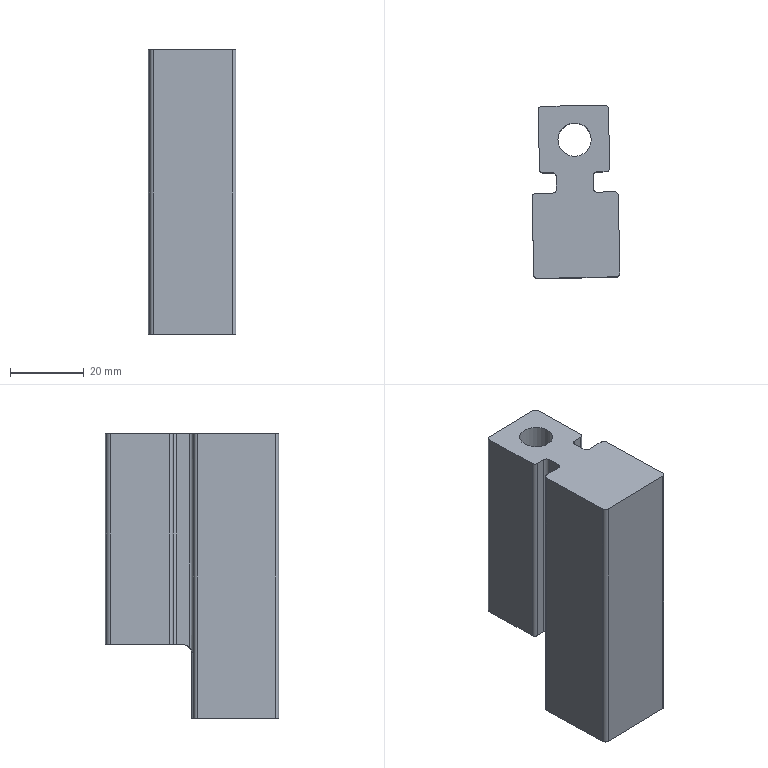Part | NX | features PU-8 2 | 1 solid | 30 faces | box 23.75 x 46.902 x 77 mm | volume 59016 mm3 | plane 15 | cylinder 15 | commonest cylinder face diameters 2 x12 6 x1 9 x1 14.5 x1
STEP:
#1=CARTESIAN_POINT('',(3034.594,-798.424,885.716));
#2=VERTEX_POINT('',#1);
#3=CARTESIAN_POINT('',(3046.592,-798.167,885.716));
#4=VERTEX_POINT('',#3);
#5=CARTESIAN_POINT('',(3046.592,-798.167,885.716));
#6=DIRECTION('',(0.9998,0.0214,0.));
#7=VECTOR('',#6,1000.);
#8=LINE('',#5,#7);
#9=EDGE_CURVE('',#2,#4,#8,.T.);
#10=ORIENTED_EDGE('',*,*,#9,.T.);
#11=CARTESIAN_POINT('',(3046.592,-798.167,945.716));
#12=VERTEX_POINT('',#11);
#13=CARTESIAN_POINT('',(3046.592,-798.167,945.716));
#14=DIRECTION('',(0.,0.,-1.));
#15=VECTOR('',#14,1000.);
#16=LINE('',#13,#15);
#17=EDGE_CURVE('',#4,#12,#16,.F.);
#18=ORIENTED_EDGE('',*,*,#17,.T.);
#19=CARTESIAN_POINT('',(3051.243,-798.068,945.716));
#20=VERTEX_POINT('',#19);
#21=CARTESIAN_POINT('',(2865.876,-802.035,945.716));
#22=DIRECTION('',(-0.9998,-0.0214,0.));
#23=VECTOR('',#22,1000.);
#24=LINE('',#21,#23);
#25=EDGE_CURVE('',#20,#12,#24,.T.);
#26=ORIENTED_EDGE('',*,*,#25,.F.);
#27=CARTESIAN_POINT('',(3051.243,-798.068,868.716));
#28=VERTEX_POINT('',#27);
#29=CARTESIAN_POINT('',(3051.243,-798.068,907.216));
#30=DIRECTION('',(0.,0.,-1.));
#31=VECTOR('',#30,1000.);
#32=LINE('',#29,#31);
#33=EDGE_CURVE('',#20,#28,#32,.T.);
#34=ORIENTED_EDGE('',*,*,#33,.T.);
#35=CARTESIAN_POINT('',(3029.943,-798.524,868.716));
#36=VERTEX_POINT('',#35);
#37=CARTESIAN_POINT('',(3028.943,-798.545,868.716));
#38=DIRECTION('',(-0.9998,-0.0214,0.));
#39=VECTOR('',#38,1000.);
#40=LINE('',#37,#39);
#41=EDGE_CURVE('',#28,#36,#40,.T.);
#42=ORIENTED_EDGE('',*,*,#41,.T.);
#43=CARTESIAN_POINT('',(3029.943,-798.524,945.716));
#44=VERTEX_POINT('',#43);
#45=CARTESIAN_POINT('',(3029.943,-798.524,907.216));
#46=DIRECTION('',(0.,0.,1.));
#47=VECTOR('',#46,1000.);
#48=LINE('',#45,#47);
#49=EDGE_CURVE('',#36,#44,#48,.T.);
#50=ORIENTED_EDGE('',*,*,#49,.T.);
#51=CARTESIAN_POINT('',(3034.594,-798.424,945.716));
#52=VERTEX_POINT('',#51);
#53=CARTESIAN_POINT('',(2865.876,-802.035,945.716));
#54=DIRECTION('',(-0.9998,-0.0214,0.));
#55=VECTOR('',#54,1000.);
#56=LINE('',#53,#55);
#57=EDGE_CURVE('',#52,#44,#56,.T.);
#58=ORIENTED_EDGE('',*,*,#57,.F.);
#59=CARTESIAN_POINT('',(3034.594,-798.424,868.716));
#60=DIRECTION('',(0.,0.,1.));
#61=VECTOR('',#60,1000.);
#62=LINE('',#59,#61);
#63=EDGE_CURVE('',#52,#2,#62,.F.);
#64=ORIENTED_EDGE('',*,*,#63,.T.);
#65=EDGE_LOOP('',(#10,#18,#26,#34,#42,#50,#58,#64));
#66=FACE_BOUND('',#65,.T.);
#67=CARTESIAN_POINT('',(3048.917,-798.117,907.216));
#68=DIRECTION('',(-0.0214,0.9998,0.));
#69=DIRECTION('',(-0.9998,-0.0214,0.));
#70=AXIS2_PLACEMENT_3D('',#67,#68,#69);
#71=PLANE('',#70);
#72=ADVANCED_FACE('',(#66),#71,.T.);
#73=CARTESIAN_POINT('',(3028.965,-799.545,868.716));
#74=VERTEX_POINT('',#73);
#75=CARTESIAN_POINT('',(3029.964,-799.523,868.716));
#76=DIRECTION('',(0.,0.,-1.));
#77=DIRECTION('',(-1.,0.,0.));
#78=AXIS2_PLACEMENT_3D('',#75,#76,#77);
#79=CIRCLE('',#78,1.);
#80=EDGE_CURVE('',#74,#36,#79,.T.);
#81=ORIENTED_EDGE('',*,*,#80,.F.);
#82=CARTESIAN_POINT('',(3028.965,-799.545,945.716));
#83=VERTEX_POINT('',#82);
#84=CARTESIAN_POINT('',(3028.965,-799.545,888.716));
#85=DIRECTION('',(0.,0.,1.));
#86=VECTOR('',#85,1000.);
#87=LINE('',#84,#86);
#88=EDGE_CURVE('',#83,#74,#87,.F.);
#89=ORIENTED_EDGE('',*,*,#88,.F.);
#90=CARTESIAN_POINT('',(3029.964,-799.523,945.716));
#91=DIRECTION('',(0.,0.,1.));
#92=DIRECTION('',(1.,0.,0.));
#93=AXIS2_PLACEMENT_3D('',#90,#91,#92);
#94=CIRCLE('',#93,1.);
#95=EDGE_CURVE('',#44,#83,#94,.T.);
#96=ORIENTED_EDGE('',*,*,#95,.F.);
#97=ORIENTED_EDGE('',*,*,#49,.F.);
#98=EDGE_LOOP('',(#81,#89,#96,#97));
#99=FACE_BOUND('',#98,.T.);
#100=CARTESIAN_POINT('',(3029.964,-799.523,907.216));
#101=DIRECTION('',(0.,0.,1.));
#102=DIRECTION('',(0.,-1.,0.));
#103=AXIS2_PLACEMENT_3D('',#100,#101,#102);
#104=CYLINDRICAL_SURFACE('',#103,1.);
#105=ADVANCED_FACE('',(#99),#104,.T.);
#106=CARTESIAN_POINT('',(3029.414,-820.542,868.716));
#107=VERTEX_POINT('',#106);
#108=CARTESIAN_POINT('',(3028.938,-798.32,868.716));
#109=DIRECTION('',(-0.0214,0.9998,0.));
#110=VECTOR('',#109,1000.);
#111=LINE('',#108,#110);
#112=EDGE_CURVE('',#107,#74,#111,.T.);
#113=ORIENTED_EDGE('',*,*,#112,.F.);
#114=CARTESIAN_POINT('',(3029.414,-820.542,945.716));
#115=VERTEX_POINT('',#114);
#116=CARTESIAN_POINT('',(3029.414,-820.542,945.716));
#117=DIRECTION('',(0.,0.,-1.));
#118=VECTOR('',#117,1000.);
#119=LINE('',#116,#118);
#120=EDGE_CURVE('',#107,#115,#119,.F.);
#121=ORIENTED_EDGE('',*,*,#120,.T.);
#122=CARTESIAN_POINT('',(3029.19,-810.082,945.716));
#123=DIRECTION('',(-0.0214,0.9998,0.));
#124=VECTOR('',#123,1000.);
#125=LINE('',#122,#124);
#126=EDGE_CURVE('',#83,#115,#125,.F.);
#127=ORIENTED_EDGE('',*,*,#126,.F.);
#128=ORIENTED_EDGE('',*,*,#88,.T.);
#129=EDGE_LOOP('',(#113,#121,#127,#128));
#130=FACE_BOUND('',#129,.T.);
#131=CARTESIAN_POINT('',(3029.19,-810.082,888.716));
#132=DIRECTION('',(-0.9998,-0.0214,0.));
#133=DIRECTION('',(0.0214,-0.9998,0.));
#134=AXIS2_PLACEMENT_3D('',#131,#132,#133);
#135=PLANE('',#134);
#136=ADVANCED_FACE('',(#130),#135,.T.);
#137=CARTESIAN_POINT('',(3030.435,-821.52,945.716));
#138=VERTEX_POINT('',#137);
#139=CARTESIAN_POINT('',(3030.414,-820.521,945.716));
#140=DIRECTION('',(0.,0.,1.));
#141=DIRECTION('',(1.,0.,0.));
#142=AXIS2_PLACEMENT_3D('',#139,#140,#141);
#143=CIRCLE('',#142,1.);
#144=EDGE_CURVE('',#115,#138,#143,.T.);
#145=ORIENTED_EDGE('',*,*,#144,.F.);
#146=ORIENTED_EDGE('',*,*,#120,.F.);
#147=CARTESIAN_POINT('',(3030.435,-821.52,868.716));
#148=VERTEX_POINT('',#147);
#149=CARTESIAN_POINT('',(3030.414,-820.521,868.716));
#150=DIRECTION('',(0.,0.,-1.));
#151=DIRECTION('',(-1.,0.,0.));
#152=AXIS2_PLACEMENT_3D('',#149,#150,#151);
#153=CIRCLE('',#152,1.);
#154=EDGE_CURVE('',#148,#107,#153,.T.);
#155=ORIENTED_EDGE('',*,*,#154,.F.);
#156=CARTESIAN_POINT('',(3030.435,-821.52,868.716));
#157=DIRECTION('',(0.,0.,-1.));
#158=VECTOR('',#157,1000.);
#159=LINE('',#156,#158);
#160=EDGE_CURVE('',#138,#148,#159,.T.);
#161=ORIENTED_EDGE('',*,*,#160,.F.);
#162=EDGE_LOOP('',(#145,#146,#155,#161));
#163=FACE_BOUND('',#162,.T.);
#164=CARTESIAN_POINT('',(3030.414,-820.521,888.716));
#165=DIRECTION('',(0.,0.,1.));
#166=DIRECTION('',(0.,-1.,0.));
#167=AXIS2_PLACEMENT_3D('',#164,#165,#166);
#168=CYLINDRICAL_SURFACE('',#167,1.);
#169=ADVANCED_FACE('',(#163),#168,.T.);
#170=CARTESIAN_POINT('',(3051.735,-821.064,868.716));
#171=VERTEX_POINT('',#170);
#172=CARTESIAN_POINT('',(3040.517,-821.305,868.716));
#173=DIRECTION('',(0.9998,0.0214,0.));
#174=VECTOR('',#173,1000.);
#175=LINE('',#172,#174);
#176=EDGE_CURVE('',#148,#171,#175,.T.);
#177=ORIENTED_EDGE('',*,*,#176,.T.);
#178=CARTESIAN_POINT('',(3051.735,-821.064,945.716));
#179=VERTEX_POINT('',#178);
#180=CARTESIAN_POINT('',(3051.735,-821.064,945.716));
#181=DIRECTION('',(0.,0.,-1.));
#182=VECTOR('',#181,1000.);
#183=LINE('',#180,#182);
#184=EDGE_CURVE('',#171,#179,#183,.F.);
#185=ORIENTED_EDGE('',*,*,#184,.T.);
#186=CARTESIAN_POINT('',(2866.368,-825.032,945.716));
#187=DIRECTION('',(-0.9998,-0.0214,0.));
#188=VECTOR('',#187,1000.);
#189=LINE('',#186,#188);
#190=EDGE_CURVE('',#138,#179,#189,.F.);
#191=ORIENTED_EDGE('',*,*,#190,.F.);
#192=ORIENTED_EDGE('',*,*,#160,.T.);
#193=EDGE_LOOP('',(#177,#185,#191,#192));
#194=FACE_BOUND('',#193,.T.);
#195=CARTESIAN_POINT('',(3029.435,-821.542,888.716));
#196=DIRECTION('',(-0.0214,0.9998,0.));
#197=DIRECTION('',(0.,0.,-1.));
#198=AXIS2_PLACEMENT_3D('',#195,#196,#197);
#199=PLANE('',#198);
#200=ADVANCED_FACE('',(#194),#199,.F.);
#201=CARTESIAN_POINT('',(3052.714,-820.043,945.716));
#202=VERTEX_POINT('',#201);
#203=CARTESIAN_POINT('',(3051.714,-820.065,945.716));
#204=DIRECTION('',(0.,0.,1.));
#205=DIRECTION('',(1.,0.,0.));
#206=AXIS2_PLACEMENT_3D('',#203,#204,#205);
#207=CIRCLE('',#206,1.);
#208=EDGE_CURVE('',#179,#202,#207,.T.);
#209=ORIENTED_EDGE('',*,*,#208,.F.);
#210=ORIENTED_EDGE('',*,*,#184,.F.);
#211=CARTESIAN_POINT('',(3052.714,-820.043,868.716));
#212=VERTEX_POINT('',#211);
#213=CARTESIAN_POINT('',(3051.714,-820.065,868.716));
#214=DIRECTION('',(0.,0.,-1.));
#215=DIRECTION('',(-1.,0.,0.));
#216=AXIS2_PLACEMENT_3D('',#213,#214,#215);
#217=CIRCLE('',#216,1.);
#218=EDGE_CURVE('',#212,#171,#217,.T.);
#219=ORIENTED_EDGE('',*,*,#218,.F.);
#220=CARTESIAN_POINT('',(3052.714,-820.043,868.716));
#221=DIRECTION('',(0.,0.,-1.));
#222=VECTOR('',#221,1000.);
#223=LINE('',#220,#222);
#224=EDGE_CURVE('',#202,#212,#223,.T.);
#225=ORIENTED_EDGE('',*,*,#224,.F.);
#226=EDGE_LOOP('',(#209,#210,#219,#225));
#227=FACE_BOUND('',#226,.T.);
#228=CARTESIAN_POINT('',(3051.714,-820.065,888.716));
#229=DIRECTION('',(0.,0.,1.));
#230=DIRECTION('',(1.,0.,0.));
#231=AXIS2_PLACEMENT_3D('',#228,#229,#230);
#232=CYLINDRICAL_SURFACE('',#231,1.);
#233=ADVANCED_FACE('',(#227),#232,.T.);
#234=CARTESIAN_POINT('',(3052.264,-799.046,868.716));
#235=VERTEX_POINT('',#234);
#236=CARTESIAN_POINT('',(3052.483,-809.276,868.716));
#237=DIRECTION('',(0.0214,-0.9998,0.));
#238=VECTOR('',#237,1000.);
#239=LINE('',#236,#238);
#240=EDGE_CURVE('',#235,#212,#239,.T.);
#241=ORIENTED_EDGE('',*,*,#240,.F.);
#242=CARTESIAN_POINT('',(3052.264,-799.046,945.716));
#243=VERTEX_POINT('',#242);
#244=CARTESIAN_POINT('',(3052.264,-799.046,888.716));
#245=DIRECTION('',(0.,0.,-1.));
#246=VECTOR('',#245,1000.);
#247=LINE('',#244,#246);
#248=EDGE_CURVE('',#235,#243,#247,.F.);
#249=ORIENTED_EDGE('',*,*,#248,.T.);
#250=CARTESIAN_POINT('',(3056.461,-995.133,945.716));
#251=DIRECTION('',(-0.0214,0.9998,0.));
#252=VECTOR('',#251,1000.);
#253=LINE('',#250,#252);
#254=EDGE_CURVE('',#243,#202,#253,.F.);
#255=ORIENTED_EDGE('',*,*,#254,.T.);
#256=ORIENTED_EDGE('',*,*,#224,.T.);
#257=EDGE_LOOP('',(#241,#249,#255,#256));
#258=FACE_BOUND('',#257,.T.);
#259=CARTESIAN_POINT('',(3052.735,-821.043,888.716));
#260=DIRECTION('',(0.9998,0.0214,0.));
#261=DIRECTION('',(0.,0.,-1.));
#262=AXIS2_PLACEMENT_3D('',#259,#260,#261);
#263=PLANE('',#262);
#264=ADVANCED_FACE('',(#258),#263,.T.);
#265=CARTESIAN_POINT('',(3051.265,-799.067,945.716));
#266=DIRECTION('',(0.,0.,1.));
#267=DIRECTION('',(1.,0.,0.));
#268=AXIS2_PLACEMENT_3D('',#265,#266,#267);
#269=CIRCLE('',#268,1.);
#270=EDGE_CURVE('',#243,#20,#269,.T.);
#271=ORIENTED_EDGE('',*,*,#270,.F.);
#272=ORIENTED_EDGE('',*,*,#248,.F.);
#273=CARTESIAN_POINT('',(3051.265,-799.067,868.716));
#274=DIRECTION('',(0.,0.,-1.));
#275=DIRECTION('',(-1.,0.,0.));
#276=AXIS2_PLACEMENT_3D('',#273,#274,#275);
#277=CIRCLE('',#276,1.);
#278=EDGE_CURVE('',#28,#235,#277,.T.);
#279=ORIENTED_EDGE('',*,*,#278,.F.);
#280=ORIENTED_EDGE('',*,*,#33,.F.);
#281=EDGE_LOOP('',(#271,#272,#279,#280));
#282=FACE_BOUND('',#281,.T.);
#283=CARTESIAN_POINT('',(3051.265,-799.067,907.216));
#284=DIRECTION('',(0.,0.,-1.));
#285=DIRECTION('',(-1.,0.,0.));
#286=AXIS2_PLACEMENT_3D('',#283,#284,#285);
#287=CYLINDRICAL_SURFACE('',#286,1.);
#288=ADVANCED_FACE('',(#282),#287,.T.);
#289=ORIENTED_EDGE('',*,*,#270,.T.);
#290=ORIENTED_EDGE('',*,*,#25,.T.);
#291=CARTESIAN_POINT('',(3045.571,-797.189,945.716));
#292=VERTEX_POINT('',#291);
#293=CARTESIAN_POINT('',(3046.57,-797.167,945.716));
#294=DIRECTION('',(0.,0.,1.));
#295=DIRECTION('',(1.,0.,0.));
#296=AXIS2_PLACEMENT_3D('',#293,#294,#295);
#297=CIRCLE('',#296,1.);
#298=EDGE_CURVE('',#12,#292,#297,.F.);
#299=ORIENTED_EDGE('',*,*,#298,.T.);
#300=CARTESIAN_POINT('',(3045.496,-793.69,945.716));
#301=VERTEX_POINT('',#300);
#302=CARTESIAN_POINT('',(3049.882,-998.642,945.716));
#303=DIRECTION('',(-0.0214,0.9998,0.));
#304=VECTOR('',#303,1000.);
#305=LINE('',#302,#304);
#306=EDGE_CURVE('',#301,#292,#305,.F.);
#307=ORIENTED_EDGE('',*,*,#306,.F.);
#308=CARTESIAN_POINT('',(3046.474,-792.668,945.716));
#309=VERTEX_POINT('',#308);
#310=CARTESIAN_POINT('',(3046.495,-793.668,945.716));
#311=DIRECTION('',(0.,0.,1.));
#312=DIRECTION('',(0.9998,0.0214,0.));
#313=AXIS2_PLACEMENT_3D('',#310,#311,#312);
#314=CIRCLE('',#313,1.);
#315=EDGE_CURVE('',#309,#301,#314,.T.);
#316=ORIENTED_EDGE('',*,*,#315,.F.);
#317=CARTESIAN_POINT('',(3048.973,-792.615,945.716));
#318=VERTEX_POINT('',#317);
#319=CARTESIAN_POINT('',(2867.193,-796.506,945.716));
#320=DIRECTION('',(0.9998,0.0214,0.));
#321=VECTOR('',#320,1000.);
#322=LINE('',#319,#321);
#323=EDGE_CURVE('',#318,#309,#322,.F.);
#324=ORIENTED_EDGE('',*,*,#323,.F.);
#325=CARTESIAN_POINT('',(3049.952,-791.594,945.716));
#326=VERTEX_POINT('',#325);
#327=CARTESIAN_POINT('',(3048.952,-791.615,945.716));
#328=DIRECTION('',(0.,0.,1.));
#329=DIRECTION('',(0.9998,0.0214,0.));
#330=AXIS2_PLACEMENT_3D('',#327,#328,#329);
#331=CIRCLE('',#330,1.);
#332=EDGE_CURVE('',#326,#318,#331,.F.);
#333=ORIENTED_EDGE('',*,*,#332,.F.);
#334=CARTESIAN_POINT('',(3049.609,-775.597,945.716));
#335=VERTEX_POINT('',#334);
#336=CARTESIAN_POINT('',(3054.392,-999.046,945.716));
#337=DIRECTION('',(-0.0214,0.9998,0.));
#338=VECTOR('',#337,1000.);
#339=LINE('',#336,#338);
#340=EDGE_CURVE('',#335,#326,#339,.F.);
#341=ORIENTED_EDGE('',*,*,#340,.F.);
#342=CARTESIAN_POINT('',(3048.588,-774.619,945.716));
#343=VERTEX_POINT('',#342);
#344=CARTESIAN_POINT('',(3048.61,-775.619,945.716));
#345=DIRECTION('',(0.,0.,1.));
#346=DIRECTION('',(0.9998,0.0214,0.));
#347=AXIS2_PLACEMENT_3D('',#344,#345,#346);
#348=CIRCLE('',#347,1.);
#349=EDGE_CURVE('',#343,#335,#348,.F.);
#350=ORIENTED_EDGE('',*,*,#349,.F.);
#351=CARTESIAN_POINT('',(3031.592,-774.983,945.716));
#352=VERTEX_POINT('',#351);
#353=CARTESIAN_POINT('',(2866.808,-778.51,945.716));
#354=DIRECTION('',(-0.9998,-0.0214,0.));
#355=VECTOR('',#354,1000.);
#356=LINE('',#353,#355);
#357=EDGE_CURVE('',#352,#343,#356,.F.);
#358=ORIENTED_EDGE('',*,*,#357,.F.);
#359=CARTESIAN_POINT('',(3030.614,-776.004,945.716));
#360=VERTEX_POINT('',#359);
#361=CARTESIAN_POINT('',(3031.614,-775.983,945.716));
#362=DIRECTION('',(0.,0.,1.));
#363=DIRECTION('',(0.9998,0.0214,0.));
#364=AXIS2_PLACEMENT_3D('',#361,#362,#363);
#365=CIRCLE('',#364,1.);
#366=EDGE_CURVE('',#360,#352,#365,.F.);
#367=ORIENTED_EDGE('',*,*,#366,.F.);
#368=CARTESIAN_POINT('',(3030.956,-792.,945.716));
#369=VERTEX_POINT('',#368);
#370=CARTESIAN_POINT('',(3035.396,-999.452,945.716));
#371=DIRECTION('',(0.0214,-0.9998,0.));
#372=VECTOR('',#371,1000.);
#373=LINE('',#370,#372);
#374=EDGE_CURVE('',#369,#360,#373,.F.);
#375=ORIENTED_EDGE('',*,*,#374,.F.);
#376=CARTESIAN_POINT('',(3031.977,-792.979,945.716));
#377=VERTEX_POINT('',#376);
#378=CARTESIAN_POINT('',(3031.956,-791.979,945.716));
#379=DIRECTION('',(0.,0.,1.));
#380=DIRECTION('',(0.9998,0.0214,0.));
#381=AXIS2_PLACEMENT_3D('',#378,#379,#380);
#382=CIRCLE('',#381,1.);
#383=EDGE_CURVE('',#377,#369,#382,.F.);
#384=ORIENTED_EDGE('',*,*,#383,.F.);
#385=CARTESIAN_POINT('',(3034.477,-792.925,945.716));
#386=VERTEX_POINT('',#385);
#387=CARTESIAN_POINT('',(2867.193,-796.506,945.716));
#388=DIRECTION('',(0.9998,0.0214,0.));
#389=VECTOR('',#388,1000.);
#390=LINE('',#387,#389);
#391=EDGE_CURVE('',#386,#377,#390,.F.);
#392=ORIENTED_EDGE('',*,*,#391,.F.);
#393=CARTESIAN_POINT('',(3035.498,-793.904,945.716));
#394=VERTEX_POINT('',#393);
#395=CARTESIAN_POINT('',(3034.498,-793.925,945.716));
#396=DIRECTION('',(0.,0.,1.));
#397=DIRECTION('',(0.9998,0.0214,0.));
#398=AXIS2_PLACEMENT_3D('',#395,#396,#397);
#399=CIRCLE('',#398,1.);
#400=EDGE_CURVE('',#394,#386,#399,.T.);
#401=ORIENTED_EDGE('',*,*,#400,.F.);
#402=CARTESIAN_POINT('',(3035.573,-797.403,945.716));
#403=VERTEX_POINT('',#402);
#404=CARTESIAN_POINT('',(3039.884,-998.856,945.716));
#405=DIRECTION('',(0.0214,-0.9998,0.));
#406=VECTOR('',#405,1000.);
#407=LINE('',#404,#406);
#408=EDGE_CURVE('',#403,#394,#407,.F.);
#409=ORIENTED_EDGE('',*,*,#408,.F.);
#410=CARTESIAN_POINT('',(3034.573,-797.424,945.716));
#411=DIRECTION('',(0.,0.,1.));
#412=DIRECTION('',(1.,0.,0.));
#413=AXIS2_PLACEMENT_3D('',#410,#411,#412);
#414=CIRCLE('',#413,1.);
#415=EDGE_CURVE('',#403,#52,#414,.F.);
#416=ORIENTED_EDGE('',*,*,#415,.T.);
#417=ORIENTED_EDGE('',*,*,#57,.T.);
#418=ORIENTED_EDGE('',*,*,#95,.T.);
#419=ORIENTED_EDGE('',*,*,#126,.T.);
#420=ORIENTED_EDGE('',*,*,#144,.T.);
#421=ORIENTED_EDGE('',*,*,#190,.T.);
#422=ORIENTED_EDGE('',*,*,#208,.T.);
#423=ORIENTED_EDGE('',*,*,#254,.F.);
#424=EDGE_LOOP('',(#289,#290,#299,#307,#316,#324,#333,#341,#350,#358,#367,#375,#384,#392,#401,#409,#416,#417,#418,#419,#420,#421,#422,#423));
#425=FACE_BOUND('',#424,.T.);
#426=CARTESIAN_POINT('',(3044.952,-783.979,945.716));
#427=VERTEX_POINT('',#426);
#428=CARTESIAN_POINT('',(3040.452,-783.979,945.716));
#429=DIRECTION('',(0.,0.,1.));
#430=DIRECTION('',(1.,0.,0.));
#431=AXIS2_PLACEMENT_3D('',#428,#429,#430);
#432=CIRCLE('',#431,4.5);
#433=EDGE_CURVE('',#427,#427,#432,.F.);
#434=ORIENTED_EDGE('',*,*,#433,.T.);
#435=EDGE_LOOP('',(#434));
#436=FACE_BOUND('',#435,.T.);
#437=CARTESIAN_POINT('',(2870.094,-999.122,945.716));
#438=DIRECTION('',(0.,0.,1.));
#439=DIRECTION('',(0.,1.,0.));
#440=AXIS2_PLACEMENT_3D('',#437,#438,#439);
#441=PLANE('',#440);
#442=ADVANCED_FACE('',(#425,#436),#441,.T.);
#443=ORIENTED_EDGE('',*,*,#41,.F.);
#444=ORIENTED_EDGE('',*,*,#278,.T.);
#445=ORIENTED_EDGE('',*,*,#240,.T.);
#446=ORIENTED_EDGE('',*,*,#218,.T.);
#447=ORIENTED_EDGE('',*,*,#176,.F.);
#448=ORIENTED_EDGE('',*,*,#154,.T.);
#449=ORIENTED_EDGE('',*,*,#112,.T.);
#450=ORIENTED_EDGE('',*,*,#80,.T.);
#451=EDGE_LOOP('',(#443,#444,#445,#446,#447,#448,#449,#450));
#452=FACE_BOUND('',#451,.T.);
#453=CARTESIAN_POINT('',(3040.266,-809.538,868.716));
#454=DIRECTION('',(0.,0.,-1.));
#455=DIRECTION('',(-0.0349,0.9994,0.));
#456=AXIS2_PLACEMENT_3D('',#453,#454,#455);
#457=PLANE('',#456);
#458=ADVANCED_FACE('',(#452),#457,.T.);
#459=ORIENTED_EDGE('',*,*,#306,.T.);
#460=CARTESIAN_POINT('',(3045.571,-797.189,887.952));
#461=VERTEX_POINT('',#460);
#462=CARTESIAN_POINT('',(3045.571,-797.189,868.716));
#463=DIRECTION('',(0.,0.,-1.));
#464=VECTOR('',#463,1000.);
#465=LINE('',#462,#464);
#466=EDGE_CURVE('',#292,#461,#465,.T.);
#467=ORIENTED_EDGE('',*,*,#466,.T.);
#468=CARTESIAN_POINT('',(3045.528,-795.189,888.716));
#469=VERTEX_POINT('',#468);
#470=CARTESIAN_POINT('',(3045.528,-795.189,885.716));
#471=DIRECTION('',(0.9998,0.0214,0.));
#472=DIRECTION('',(-0.0214,0.9998,0.));
#473=AXIS2_PLACEMENT_3D('',#470,#471,#472);
#474=CIRCLE('',#473,3.);
#475=EDGE_CURVE('',#461,#469,#474,.F.);
#476=ORIENTED_EDGE('',*,*,#475,.T.);
#477=CARTESIAN_POINT('',(3045.496,-793.69,888.716));
#478=VERTEX_POINT('',#477);
#479=CARTESIAN_POINT('',(3045.832,-809.419,888.716));
#480=DIRECTION('',(0.0214,-0.9998,0.));
#481=VECTOR('',#480,1000.);
#482=LINE('',#479,#481);
#483=EDGE_CURVE('',#478,#469,#482,.T.);
#484=ORIENTED_EDGE('',*,*,#483,.F.);
#485=CARTESIAN_POINT('',(3045.496,-793.69,900.716));
#486=DIRECTION('',(0.,0.,-1.));
#487=VECTOR('',#486,1000.);
#488=LINE('',#485,#487);
#489=EDGE_CURVE('',#301,#478,#488,.T.);
#490=ORIENTED_EDGE('',*,*,#489,.F.);
#491=EDGE_LOOP('',(#459,#467,#476,#484,#490));
#492=FACE_BOUND('',#491,.T.);
#493=CARTESIAN_POINT('',(3045.485,-793.19,900.716));
#494=DIRECTION('',(0.9998,0.0214,0.));
#495=DIRECTION('',(-0.0214,0.9998,0.));
#496=AXIS2_PLACEMENT_3D('',#493,#494,#495);
#497=PLANE('',#496);
#498=ADVANCED_FACE('',(#492),#497,.T.);
#499=ORIENTED_EDGE('',*,*,#298,.F.);
#500=ORIENTED_EDGE('',*,*,#17,.F.);
#501=CARTESIAN_POINT('',(3045.571,-797.189,887.952));
#502=CARTESIAN_POINT('',(3045.578,-797.534,887.644));
#503=CARTESIAN_POINT('',(3045.906,-798.032,886.9));
#504=CARTESIAN_POINT('',(3046.363,-798.172,886.113));
#505=CARTESIAN_POINT('',(3046.592,-798.167,885.716));
#506=B_SPLINE_CURVE_WITH_KNOTS('',3,(#501,#502,#503,#504,#505),.UNSPECIFIED.,.F.,.F.,(4,1,4),(0.,0.001374,0.002748),.UNSPECIFIED.);
#507=EDGE_CURVE('',#4,#461,#506,.F.);
#508=ORIENTED_EDGE('',*,*,#507,.T.);
#509=ORIENTED_EDGE('',*,*,#466,.F.);
#510=EDGE_LOOP('',(#499,#500,#508,#509));
#511=FACE_BOUND('',#510,.T.);
#512=CARTESIAN_POINT('',(3046.57,-797.167,900.716));
#513=DIRECTION('',(0.,0.,1.));
#514=DIRECTION('',(1.,0.,0.));
#515=AXIS2_PLACEMENT_3D('',#512,#513,#514);
#516=CYLINDRICAL_SURFACE('',#515,1.);
#517=ADVANCED_FACE('',(#511),#516,.F.);
#518=CARTESIAN_POINT('',(3035.573,-797.403,887.952));
#519=VERTEX_POINT('',#518);
#520=CARTESIAN_POINT('',(3035.573,-797.403,945.716));
#521=DIRECTION('',(0.,0.,1.));
#522=VECTOR('',#521,1000.);
#523=LINE('',#520,#522);
#524=EDGE_CURVE('',#519,#403,#523,.T.);
#525=ORIENTED_EDGE('',*,*,#524,.F.);
#526=CARTESIAN_POINT('',(3035.573,-797.403,887.952));
#527=CARTESIAN_POINT('',(3035.58,-797.748,887.644));
#528=CARTESIAN_POINT('',(3035.274,-798.259,886.9));
#529=CARTESIAN_POINT('',(3034.823,-798.419,886.113));
#530=CARTESIAN_POINT('',(3034.594,-798.424,885.716));
#531=B_SPLINE_CURVE_WITH_KNOTS('',3,(#526,#527,#528,#529,#530),.UNSPECIFIED.,.F.,.F.,(4,1,4),(0.,0.001374,0.002748),.UNSPECIFIED.);
#532=EDGE_CURVE('',#519,#2,#531,.T.);
#533=ORIENTED_EDGE('',*,*,#532,.T.);
#534=ORIENTED_EDGE('',*,*,#63,.F.);
#535=ORIENTED_EDGE('',*,*,#415,.F.);
#536=EDGE_LOOP('',(#525,#533,#534,#535));
#537=FACE_BOUND('',#536,.T.);
#538=CARTESIAN_POINT('',(3034.573,-797.424,900.716));
#539=DIRECTION('',(0.,0.,-1.));
#540=DIRECTION('',(-1.,0.,0.));
#541=AXIS2_PLACEMENT_3D('',#538,#539,#540);
#542=CYLINDRICAL_SURFACE('',#541,1.);
#543=ADVANCED_FACE('',(#537),#542,.F.);
#544=CARTESIAN_POINT('',(3035.53,-795.403,888.716));
#545=VERTEX_POINT('',#544);
#546=CARTESIAN_POINT('',(3035.498,-793.904,888.716));
#547=VERTEX_POINT('',#546);
#548=CARTESIAN_POINT('',(3035.835,-809.633,888.716));
#549=DIRECTION('',(-0.0214,0.9998,0.));
#550=VECTOR('',#549,1000.);
#551=LINE('',#548,#550);
#552=EDGE_CURVE('',#545,#547,#551,.T.);
#553=ORIENTED_EDGE('',*,*,#552,.F.);
#554=CARTESIAN_POINT('',(3035.53,-795.403,885.716));
#555=DIRECTION('',(-0.9998,-0.0214,0.));
#556=DIRECTION('',(0.0214,-0.9998,0.));
#557=AXIS2_PLACEMENT_3D('',#554,#555,#556);
#558=CIRCLE('',#557,3.);
#559=EDGE_CURVE('',#545,#519,#558,.F.);
#560=ORIENTED_EDGE('',*,*,#559,.T.);
#561=ORIENTED_EDGE('',*,*,#524,.T.);
#562=ORIENTED_EDGE('',*,*,#408,.T.);
#563=CARTESIAN_POINT('',(3035.498,-793.904,900.716));
#564=DIRECTION('',(0.,0.,1.));
#565=VECTOR('',#564,1000.);
#566=LINE('',#563,#565);
#567=EDGE_CURVE('',#394,#547,#566,.F.);
#568=ORIENTED_EDGE('',*,*,#567,.T.);
#569=EDGE_LOOP('',(#553,#560,#561,#562,#568));
#570=FACE_BOUND('',#569,.T.);
#571=CARTESIAN_POINT('',(3035.573,-797.403,900.716));
#572=DIRECTION('',(-0.9998,-0.0214,0.));
#573=DIRECTION('',(0.0214,-0.9998,0.));
#574=AXIS2_PLACEMENT_3D('',#571,#572,#573);
#575=PLANE('',#574);
#576=ADVANCED_FACE('',(#570),#575,.T.);
#577=ORIENTED_EDGE('',*,*,#483,.T.);
#578=CARTESIAN_POINT('',(3034.53,-795.425,888.716));
#579=DIRECTION('',(0.9998,0.0214,0.));
#580=VECTOR('',#579,1000.);
#581=LINE('',#578,#580);
#582=EDGE_CURVE('',#469,#545,#581,.F.);
#583=ORIENTED_EDGE('',*,*,#582,.T.);
#584=ORIENTED_EDGE('',*,*,#552,.T.);
#585=CARTESIAN_POINT('',(3034.477,-792.925,888.716));
#586=VERTEX_POINT('',#585);
#587=CARTESIAN_POINT('',(3034.498,-793.925,888.716));
#588=DIRECTION('',(0.,0.,-1.));
#589=DIRECTION('',(-1.,0.,0.));
#590=AXIS2_PLACEMENT_3D('',#587,#588,#589);
#591=CIRCLE('',#590,1.);
#592=EDGE_CURVE('',#547,#586,#591,.F.);
#593=ORIENTED_EDGE('',*,*,#592,.T.);
#594=CARTESIAN_POINT('',(3031.977,-792.979,888.716));
#595=VERTEX_POINT('',#594);
#596=CARTESIAN_POINT('',(3039.908,-792.809,888.716));
#597=DIRECTION('',(-0.9998,-0.0214,0.));
#598=VECTOR('',#597,1000.);
#599=LINE('',#596,#598);
#600=EDGE_CURVE('',#586,#595,#599,.T.);
#601=ORIENTED_EDGE('',*,*,#600,.T.);
#602=CARTESIAN_POINT('',(3030.956,-792.,888.716));
#603=VERTEX_POINT('',#602);
#604=CARTESIAN_POINT('',(3031.956,-791.979,888.716));
#605=DIRECTION('',(0.,0.,-1.));
#606=DIRECTION('',(-1.,0.,0.));
#607=AXIS2_PLACEMENT_3D('',#604,#605,#606);
#608=CIRCLE('',#607,1.);
#609=EDGE_CURVE('',#595,#603,#608,.T.);
#610=ORIENTED_EDGE('',*,*,#609,.T.);
#611=CARTESIAN_POINT('',(3030.614,-776.004,888.716));
#612=VERTEX_POINT('',#611);
#613=CARTESIAN_POINT('',(3031.336,-809.729,888.716));
#614=DIRECTION('',(-0.0214,0.9998,0.));
#615=VECTOR('',#614,1000.);
#616=LINE('',#613,#615);
#617=EDGE_CURVE('',#603,#612,#616,.T.);
#618=ORIENTED_EDGE('',*,*,#617,.T.);
#619=CARTESIAN_POINT('',(3031.592,-774.983,888.716));
#620=VERTEX_POINT('',#619);
#621=CARTESIAN_POINT('',(3031.614,-775.983,888.716));
#622=DIRECTION('',(0.,0.,-1.));
#623=DIRECTION('',(-1.,0.,0.));
#624=AXIS2_PLACEMENT_3D('',#621,#622,#623);
#625=CIRCLE('',#624,1.);
#626=EDGE_CURVE('',#612,#620,#625,.T.);
#627=ORIENTED_EDGE('',*,*,#626,.T.);
#628=CARTESIAN_POINT('',(3048.588,-774.619,888.716));
#629=VERTEX_POINT('',#628);
#630=CARTESIAN_POINT('',(3039.522,-774.813,888.716));
#631=DIRECTION('',(0.9998,0.0214,0.));
#632=VECTOR('',#631,1000.);
#633=LINE('',#630,#632);
#634=EDGE_CURVE('',#620,#629,#633,.T.);
#635=ORIENTED_EDGE('',*,*,#634,.T.);
#636=CARTESIAN_POINT('',(3049.609,-775.597,888.716));
#637=VERTEX_POINT('',#636);
#638=CARTESIAN_POINT('',(3048.61,-775.619,888.716));
#639=DIRECTION('',(0.,0.,-1.));
#640=DIRECTION('',(-1.,0.,0.));
#641=AXIS2_PLACEMENT_3D('',#638,#639,#640);
#642=CIRCLE('',#641,1.);
#643=EDGE_CURVE('',#629,#637,#642,.T.);
#644=ORIENTED_EDGE('',*,*,#643,.T.);
#645=CARTESIAN_POINT('',(3049.952,-791.594,888.716));
#646=VERTEX_POINT('',#645);
#647=CARTESIAN_POINT('',(3050.331,-809.323,888.716));
#648=DIRECTION('',(0.0214,-0.9998,0.));
#649=VECTOR('',#648,1000.);
#650=LINE('',#647,#649);
#651=EDGE_CURVE('',#637,#646,#650,.T.);
#652=ORIENTED_EDGE('',*,*,#651,.T.);
#653=CARTESIAN_POINT('',(3048.973,-792.615,888.716));
#654=VERTEX_POINT('',#653);
#655=CARTESIAN_POINT('',(3048.952,-791.615,888.716));
#656=DIRECTION('',(0.,0.,-1.));
#657=DIRECTION('',(-1.,0.,0.));
#658=AXIS2_PLACEMENT_3D('',#655,#656,#657);
#659=CIRCLE('',#658,1.);
#660=EDGE_CURVE('',#646,#654,#659,.T.);
#661=ORIENTED_EDGE('',*,*,#660,.T.);
#662=CARTESIAN_POINT('',(3046.474,-792.668,888.716));
#663=VERTEX_POINT('',#662);
#664=CARTESIAN_POINT('',(3039.908,-792.809,888.716));
#665=DIRECTION('',(-0.9998,-0.0214,0.));
#666=VECTOR('',#665,1000.);
#667=LINE('',#664,#666);
#668=EDGE_CURVE('',#654,#663,#667,.T.);
#669=ORIENTED_EDGE('',*,*,#668,.T.);
#670=CARTESIAN_POINT('',(3046.495,-793.668,888.716));
#671=DIRECTION('',(0.,0.,-1.));
#672=DIRECTION('',(-1.,0.,0.));
#673=AXIS2_PLACEMENT_3D('',#670,#671,#672);
#674=CIRCLE('',#673,1.);
#675=EDGE_CURVE('',#663,#478,#674,.F.);
#676=ORIENTED_EDGE('',*,*,#675,.T.);
#677=EDGE_LOOP('',(#577,#583,#584,#593,#601,#610,#618,#627,#635,#644,#652,#661,#669,#676));
#678=FACE_BOUND('',#677,.T.);
#679=CARTESIAN_POINT('',(3033.202,-783.979,888.716));
#680=VERTEX_POINT('',#679);
#681=CARTESIAN_POINT('',(3040.452,-783.979,888.716));
#682=DIRECTION('',(0.,0.,-1.));
#683=DIRECTION('',(-1.,0.,0.));
#684=AXIS2_PLACEMENT_3D('',#681,#682,#683);
#685=CIRCLE('',#684,7.25);
#686=EDGE_CURVE('',#680,#680,#685,.T.);
#687=ORIENTED_EDGE('',*,*,#686,.F.);
#688=EDGE_LOOP('',(#687));
#689=FACE_BOUND('',#688,.T.);
#690=CARTESIAN_POINT('',(3040.266,-809.538,888.716));
#691=DIRECTION('',(0.,0.,-1.));
#692=DIRECTION('',(-0.0349,0.9994,0.));
#693=AXIS2_PLACEMENT_3D('',#690,#691,#692);
#694=PLANE('',#693);
#695=ADVANCED_FACE('',(#678,#689),#694,.T.);
#696=ORIENTED_EDGE('',*,*,#592,.F.);
#697=ORIENTED_EDGE('',*,*,#567,.F.);
#698=ORIENTED_EDGE('',*,*,#400,.T.);
#699=CARTESIAN_POINT('',(3034.477,-792.925,900.716));
#700=DIRECTION('',(0.,0.,-1.));
#701=VECTOR('',#700,1000.);
#702=LINE('',#699,#701);
#703=EDGE_CURVE('',#386,#586,#702,.T.);
#704=ORIENTED_EDGE('',*,*,#703,.T.);
#705=EDGE_LOOP('',(#696,#697,#698,#704));
#706=FACE_BOUND('',#705,.T.);
#707=CARTESIAN_POINT('',(3034.498,-793.925,900.716));
#708=DIRECTION('',(0.,0.,-1.));
#709=DIRECTION('',(-0.0135,-0.9999,0.));
#710=AXIS2_PLACEMENT_3D('',#707,#708,#709);
#711=CYLINDRICAL_SURFACE('',#710,1.);
#712=ADVANCED_FACE('',(#706),#711,.F.);
#713=ORIENTED_EDGE('',*,*,#675,.F.);
#714=CARTESIAN_POINT('',(3046.474,-792.668,900.716));
#715=DIRECTION('',(0.,0.,-1.));
#716=VECTOR('',#715,1000.);
#717=LINE('',#714,#716);
#718=EDGE_CURVE('',#309,#663,#717,.T.);
#719=ORIENTED_EDGE('',*,*,#718,.F.);
#720=ORIENTED_EDGE('',*,*,#315,.T.);
#721=ORIENTED_EDGE('',*,*,#489,.T.);
#722=EDGE_LOOP('',(#713,#719,#720,#721));
#723=FACE_BOUND('',#722,.T.);
#724=CARTESIAN_POINT('',(3046.495,-793.668,900.716));
#725=DIRECTION('',(0.,0.,-1.));
#726=DIRECTION('',(-0.0135,-0.9999,0.));
#727=AXIS2_PLACEMENT_3D('',#724,#725,#726);
#728=CYLINDRICAL_SURFACE('',#727,1.);
#729=ADVANCED_FACE('',(#723),#728,.F.);
#730=ORIENTED_EDGE('',*,*,#703,.F.);
#731=ORIENTED_EDGE('',*,*,#391,.T.);
#732=CARTESIAN_POINT('',(3031.977,-792.979,900.716));
#733=DIRECTION('',(0.,0.,-1.));
#734=VECTOR('',#733,1000.);
#735=LINE('',#732,#734);
#736=EDGE_CURVE('',#377,#595,#735,.T.);
#737=ORIENTED_EDGE('',*,*,#736,.T.);
#738=ORIENTED_EDGE('',*,*,#600,.F.);
#739=EDGE_LOOP('',(#730,#731,#737,#738));
#740=FACE_BOUND('',#739,.T.);
#741=CARTESIAN_POINT('',(3050.473,-792.583,900.716));
#742=DIRECTION('',(0.0214,-0.9998,0.));
#743=DIRECTION('',(0.9998,0.0214,0.));
#744=AXIS2_PLACEMENT_3D('',#741,#742,#743);
#745=PLANE('',#744);
#746=ADVANCED_FACE('',(#740),#745,.T.);
#747=ORIENTED_EDGE('',*,*,#626,.F.);
#748=CARTESIAN_POINT('',(3030.614,-776.004,900.716));
#749=DIRECTION('',(0.,0.,-1.));
#750=VECTOR('',#749,1000.);
#751=LINE('',#748,#750);
#752=EDGE_CURVE('',#360,#612,#751,.T.);
#753=ORIENTED_EDGE('',*,*,#752,.F.);
#754=ORIENTED_EDGE('',*,*,#366,.T.);
#755=CARTESIAN_POINT('',(3031.592,-774.983,900.716));
#756=DIRECTION('',(0.,0.,-1.));
#757=VECTOR('',#756,1000.);
#758=LINE('',#755,#757);
#759=EDGE_CURVE('',#352,#620,#758,.T.);
#760=ORIENTED_EDGE('',*,*,#759,.T.);
#761=EDGE_LOOP('',(#747,#753,#754,#760));
#762=FACE_BOUND('',#761,.T.);
#763=CARTESIAN_POINT('',(3031.614,-775.983,900.716));
#764=DIRECTION('',(0.,0.,-1.));
#765=DIRECTION('',(-0.0135,-0.9999,0.));
#766=AXIS2_PLACEMENT_3D('',#763,#764,#765);
#767=CYLINDRICAL_SURFACE('',#766,1.);
#768=ADVANCED_FACE('',(#762),#767,.T.);
#769=ORIENTED_EDGE('',*,*,#634,.F.);
#770=ORIENTED_EDGE('',*,*,#759,.F.);
#771=ORIENTED_EDGE('',*,*,#357,.T.);
#772=CARTESIAN_POINT('',(3048.588,-774.619,900.716));
#773=DIRECTION('',(0.,0.,-1.));
#774=VECTOR('',#773,1000.);
#775=LINE('',#772,#774);
#776=EDGE_CURVE('',#343,#629,#775,.T.);
#777=ORIENTED_EDGE('',*,*,#776,.T.);
#778=EDGE_LOOP('',(#769,#770,#771,#777));
#779=FACE_BOUND('',#778,.T.);
#780=CARTESIAN_POINT('',(3030.093,-775.015,900.716));
#781=DIRECTION('',(-0.0214,0.9998,0.));
#782=DIRECTION('',(-0.9998,-0.0214,0.));
#783=AXIS2_PLACEMENT_3D('',#780,#781,#782);
#784=PLANE('',#783);
#785=ADVANCED_FACE('',(#779),#784,.T.);
#786=ORIENTED_EDGE('',*,*,#643,.F.);
#787=ORIENTED_EDGE('',*,*,#776,.F.);
#788=ORIENTED_EDGE('',*,*,#349,.T.);
#789=CARTESIAN_POINT('',(3049.609,-775.597,900.716));
#790=DIRECTION('',(0.,0.,-1.));
#791=VECTOR('',#790,1000.);
#792=LINE('',#789,#791);
#793=EDGE_CURVE('',#335,#637,#792,.T.);
#794=ORIENTED_EDGE('',*,*,#793,.T.);
#795=EDGE_LOOP('',(#786,#787,#788,#794));
#796=FACE_BOUND('',#795,.T.);
#797=CARTESIAN_POINT('',(3048.61,-775.619,900.716));
#798=DIRECTION('',(0.,0.,-1.));
#799=DIRECTION('',(-0.0135,-0.9999,0.));
#800=AXIS2_PLACEMENT_3D('',#797,#798,#799);
#801=CYLINDRICAL_SURFACE('',#800,1.);
#802=ADVANCED_FACE('',(#796),#801,.T.);
#803=ORIENTED_EDGE('',*,*,#651,.F.);
#804=ORIENTED_EDGE('',*,*,#793,.F.);
#805=ORIENTED_EDGE('',*,*,#340,.T.);
#806=CARTESIAN_POINT('',(3049.952,-791.594,900.716));
#807=DIRECTION('',(0.,0.,-1.));
#808=VECTOR('',#807,1000.);
#809=LINE('',#806,#808);
#810=EDGE_CURVE('',#326,#646,#809,.T.);
#811=ORIENTED_EDGE('',*,*,#810,.T.);
#812=EDGE_LOOP('',(#803,#804,#805,#811));
#813=FACE_BOUND('',#812,.T.);
#814=CARTESIAN_POINT('',(3049.866,-787.595,900.716));
#815=DIRECTION('',(0.9998,0.0214,0.));
#816=DIRECTION('',(-0.0214,0.9998,0.));
#817=AXIS2_PLACEMENT_3D('',#814,#815,#816);
#818=PLANE('',#817);
#819=ADVANCED_FACE('',(#813),#818,.T.);
#820=ORIENTED_EDGE('',*,*,#660,.F.);
#821=ORIENTED_EDGE('',*,*,#810,.F.);
#822=ORIENTED_EDGE('',*,*,#332,.T.);
#823=CARTESIAN_POINT('',(3048.973,-792.615,900.716));
#824=DIRECTION('',(0.,0.,-1.));
#825=VECTOR('',#824,1000.);
#826=LINE('',#823,#825);
#827=EDGE_CURVE('',#318,#654,#826,.T.);
#828=ORIENTED_EDGE('',*,*,#827,.T.);
#829=EDGE_LOOP('',(#820,#821,#822,#828));
#830=FACE_BOUND('',#829,.T.);
#831=CARTESIAN_POINT('',(3048.952,-791.615,900.716));
#832=DIRECTION('',(0.,0.,-1.));
#833=DIRECTION('',(-0.0135,-0.9999,0.));
#834=AXIS2_PLACEMENT_3D('',#831,#832,#833);
#835=CYLINDRICAL_SURFACE('',#834,1.);
#836=ADVANCED_FACE('',(#830),#835,.T.);
#837=ORIENTED_EDGE('',*,*,#323,.T.);
#838=ORIENTED_EDGE('',*,*,#718,.T.);
#839=ORIENTED_EDGE('',*,*,#668,.F.);
#840=ORIENTED_EDGE('',*,*,#827,.F.);
#841=EDGE_LOOP('',(#837,#838,#839,#840));
#842=FACE_BOUND('',#841,.T.);
#843=CARTESIAN_POINT('',(3050.473,-792.583,900.716));
#844=DIRECTION('',(0.0214,-0.9998,0.));
#845=DIRECTION('',(0.9998,0.0214,0.));
#846=AXIS2_PLACEMENT_3D('',#843,#844,#845);
#847=PLANE('',#846);
#848=ADVANCED_FACE('',(#842),#847,.T.);
#849=ORIENTED_EDGE('',*,*,#609,.F.);
#850=ORIENTED_EDGE('',*,*,#736,.F.);
#851=ORIENTED_EDGE('',*,*,#383,.T.);
#852=CARTESIAN_POINT('',(3030.956,-792.,900.716));
#853=DIRECTION('',(0.,0.,-1.));
#854=VECTOR('',#853,1000.);
#855=LINE('',#852,#854);
#856=EDGE_CURVE('',#369,#603,#855,.T.);
#857=ORIENTED_EDGE('',*,*,#856,.T.);
#858=EDGE_LOOP('',(#849,#850,#851,#857));
#859=FACE_BOUND('',#858,.T.);
#860=CARTESIAN_POINT('',(3031.956,-791.979,900.716));
#861=DIRECTION('',(0.,0.,-1.));
#862=DIRECTION('',(-0.0135,-0.9999,0.));
#863=AXIS2_PLACEMENT_3D('',#860,#861,#862);
#864=CYLINDRICAL_SURFACE('',#863,1.);
#865=ADVANCED_FACE('',(#859),#864,.T.);
#866=ORIENTED_EDGE('',*,*,#617,.F.);
#867=ORIENTED_EDGE('',*,*,#856,.F.);
#868=ORIENTED_EDGE('',*,*,#374,.T.);
#869=ORIENTED_EDGE('',*,*,#752,.T.);
#870=EDGE_LOOP('',(#866,#867,#868,#869));
#871=FACE_BOUND('',#870,.T.);
#872=CARTESIAN_POINT('',(3030.956,-792.,900.716));
#873=DIRECTION('',(-0.9998,-0.0214,0.));
#874=DIRECTION('',(0.0214,-0.9998,0.));
#875=AXIS2_PLACEMENT_3D('',#872,#873,#874);
#876=PLANE('',#875);
#877=ADVANCED_FACE('',(#871),#876,.T.);
#878=CARTESIAN_POINT('',(3035.952,-783.979,900.716));
#879=VERTEX_POINT('',#878);
#880=CARTESIAN_POINT('',(3040.452,-783.979,900.716));
#881=DIRECTION('',(0.,0.,-1.));
#882=DIRECTION('',(-1.,0.,0.));
#883=AXIS2_PLACEMENT_3D('',#880,#881,#882);
#884=CIRCLE('',#883,4.5);
#885=EDGE_CURVE('',#879,#879,#884,.T.);
#886=ORIENTED_EDGE('',*,*,#885,.T.);
#887=EDGE_LOOP('',(#886));
#888=FACE_BOUND('',#887,.T.);
#889=ORIENTED_EDGE('',*,*,#433,.F.);
#890=EDGE_LOOP('',(#889));
#891=FACE_BOUND('',#890,.T.);
#892=CARTESIAN_POINT('',(3040.452,-783.979,946.716));
#893=DIRECTION('',(0.,0.,-1.));
#894=DIRECTION('',(-1.,0.,0.));
#895=AXIS2_PLACEMENT_3D('',#892,#893,#894);
#896=CYLINDRICAL_SURFACE('',#895,4.5);
#897=ADVANCED_FACE('',(#888,#891),#896,.F.);
#898=ORIENTED_EDGE('',*,*,#686,.T.);
#899=EDGE_LOOP('',(#898));
#900=FACE_BOUND('',#899,.T.);
#901=CARTESIAN_POINT('',(3033.202,-783.979,900.716));
#902=VERTEX_POINT('',#901);
#903=CARTESIAN_POINT('',(3040.452,-783.979,900.716));
#904=DIRECTION('',(0.,0.,-1.));
#905=DIRECTION('',(-1.,0.,0.));
#906=AXIS2_PLACEMENT_3D('',#903,#904,#905);
#907=CIRCLE('',#906,7.25);
#908=EDGE_CURVE('',#902,#902,#907,.F.);
#909=ORIENTED_EDGE('',*,*,#908,.T.);
#910=EDGE_LOOP('',(#909));
#911=FACE_BOUND('',#910,.T.);
#912=CARTESIAN_POINT('',(3040.452,-783.979,895.716));
#913=DIRECTION('',(0.,0.,-1.));
#914=DIRECTION('',(-1.,0.,0.));
#915=AXIS2_PLACEMENT_3D('',#912,#913,#914);
#916=CYLINDRICAL_SURFACE('',#915,7.25);
#917=ADVANCED_FACE('',(#900,#911),#916,.F.);
#918=ORIENTED_EDGE('',*,*,#885,.F.);
#919=EDGE_LOOP('',(#918));
#920=FACE_BOUND('',#919,.T.);
#921=ORIENTED_EDGE('',*,*,#908,.F.);
#922=EDGE_LOOP('',(#921));
#923=FACE_BOUND('',#922,.T.);
#924=CARTESIAN_POINT('',(3040.452,-783.979,900.716));
#925=DIRECTION('',(0.,0.,-1.));
#926=DIRECTION('',(-1.,0.,0.));
#927=AXIS2_PLACEMENT_3D('',#924,#925,#926);
#928=PLANE('',#927);
#929=ADVANCED_FACE('',(#920,#923),#928,.T.);
#930=ORIENTED_EDGE('',*,*,#559,.F.);
#931=ORIENTED_EDGE('',*,*,#582,.F.);
#932=ORIENTED_EDGE('',*,*,#475,.F.);
#933=ORIENTED_EDGE('',*,*,#507,.F.);
#934=ORIENTED_EDGE('',*,*,#9,.F.);
#935=ORIENTED_EDGE('',*,*,#532,.F.);
#936=EDGE_LOOP('',(#930,#931,#932,#933,#934,#935));
#937=FACE_BOUND('',#936,.T.);
#938=CARTESIAN_POINT('',(3048.853,-795.118,885.716));
#939=DIRECTION('',(-0.9998,-0.0214,0.));
#940=DIRECTION('',(0.0214,-0.9998,0.));
#941=AXIS2_PLACEMENT_3D('',#938,#939,#940);
#942=CYLINDRICAL_SURFACE('',#941,3.);
#943=ADVANCED_FACE('',(#937),#942,.F.);
#944=CLOSED_SHELL('',(#72,#105,#136,#169,#200,#233,#264,#288,#442,#458,#498,#517,#543,#576,#695,#712,#729,#746,#768,#785,#802,#819,#836,#848,#865,#877,#897,#917,#929,#943));
#945=MANIFOLD_SOLID_BREP('',#944);
#946=(LENGTH_UNIT()NAMED_UNIT(*)SI_UNIT(.MILLI.,.METRE.));
#947=UNCERTAINTY_MEASURE_WITH_UNIT(LENGTH_MEASURE(0.0508),#946,'','');
#948=(NAMED_UNIT(*)PLANE_ANGLE_UNIT()SI_UNIT($,.RADIAN.));
#949=(NAMED_UNIT(*)SI_UNIT($,.STERADIAN.)SOLID_ANGLE_UNIT());
#950=(GEOMETRIC_REPRESENTATION_CONTEXT(3)GLOBAL_UNCERTAINTY_ASSIGNED_CONTEXT((#947))GLOBAL_UNIT_ASSIGNED_CONTEXT((#946,#948,#949))REPRESENTATION_CONTEXT('',''));
#951=ADVANCED_BREP_SHAPE_REPRESENTATION('',(#945),#950);